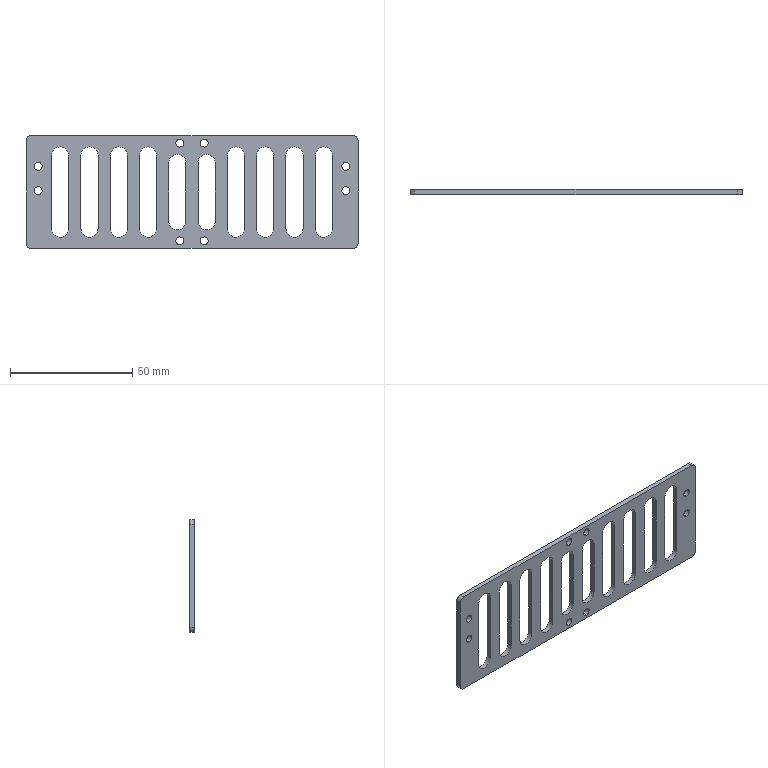Part | SolidWorks | features Extrusion 1, Fillet 1, ICE 1 | 1 solid | 76 faces | box 136 x 2 x 46 mm | volume 7575 mm3 | cylinder 50 | plane 26 | commonest cylinder face diameters 7 x30 3.2 x16 4 x4